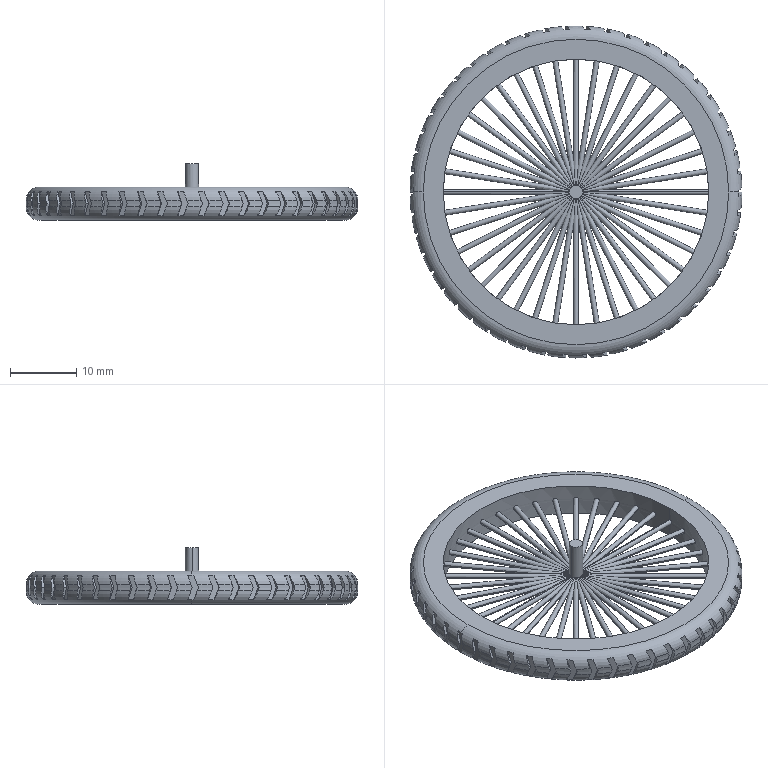Part | SolidWorks | features ICE 8, CirPattern 2, Extrusion 1, Fillet 1 | 1 solid | 394 faces | box 50 x 50 x 8.5 mm | volume 3543 mm3 | plane 254 | cylinder 136 | torus 4 | commonest cylinder face diameters 0.75 x80 50 x50 2 x4 40 x2